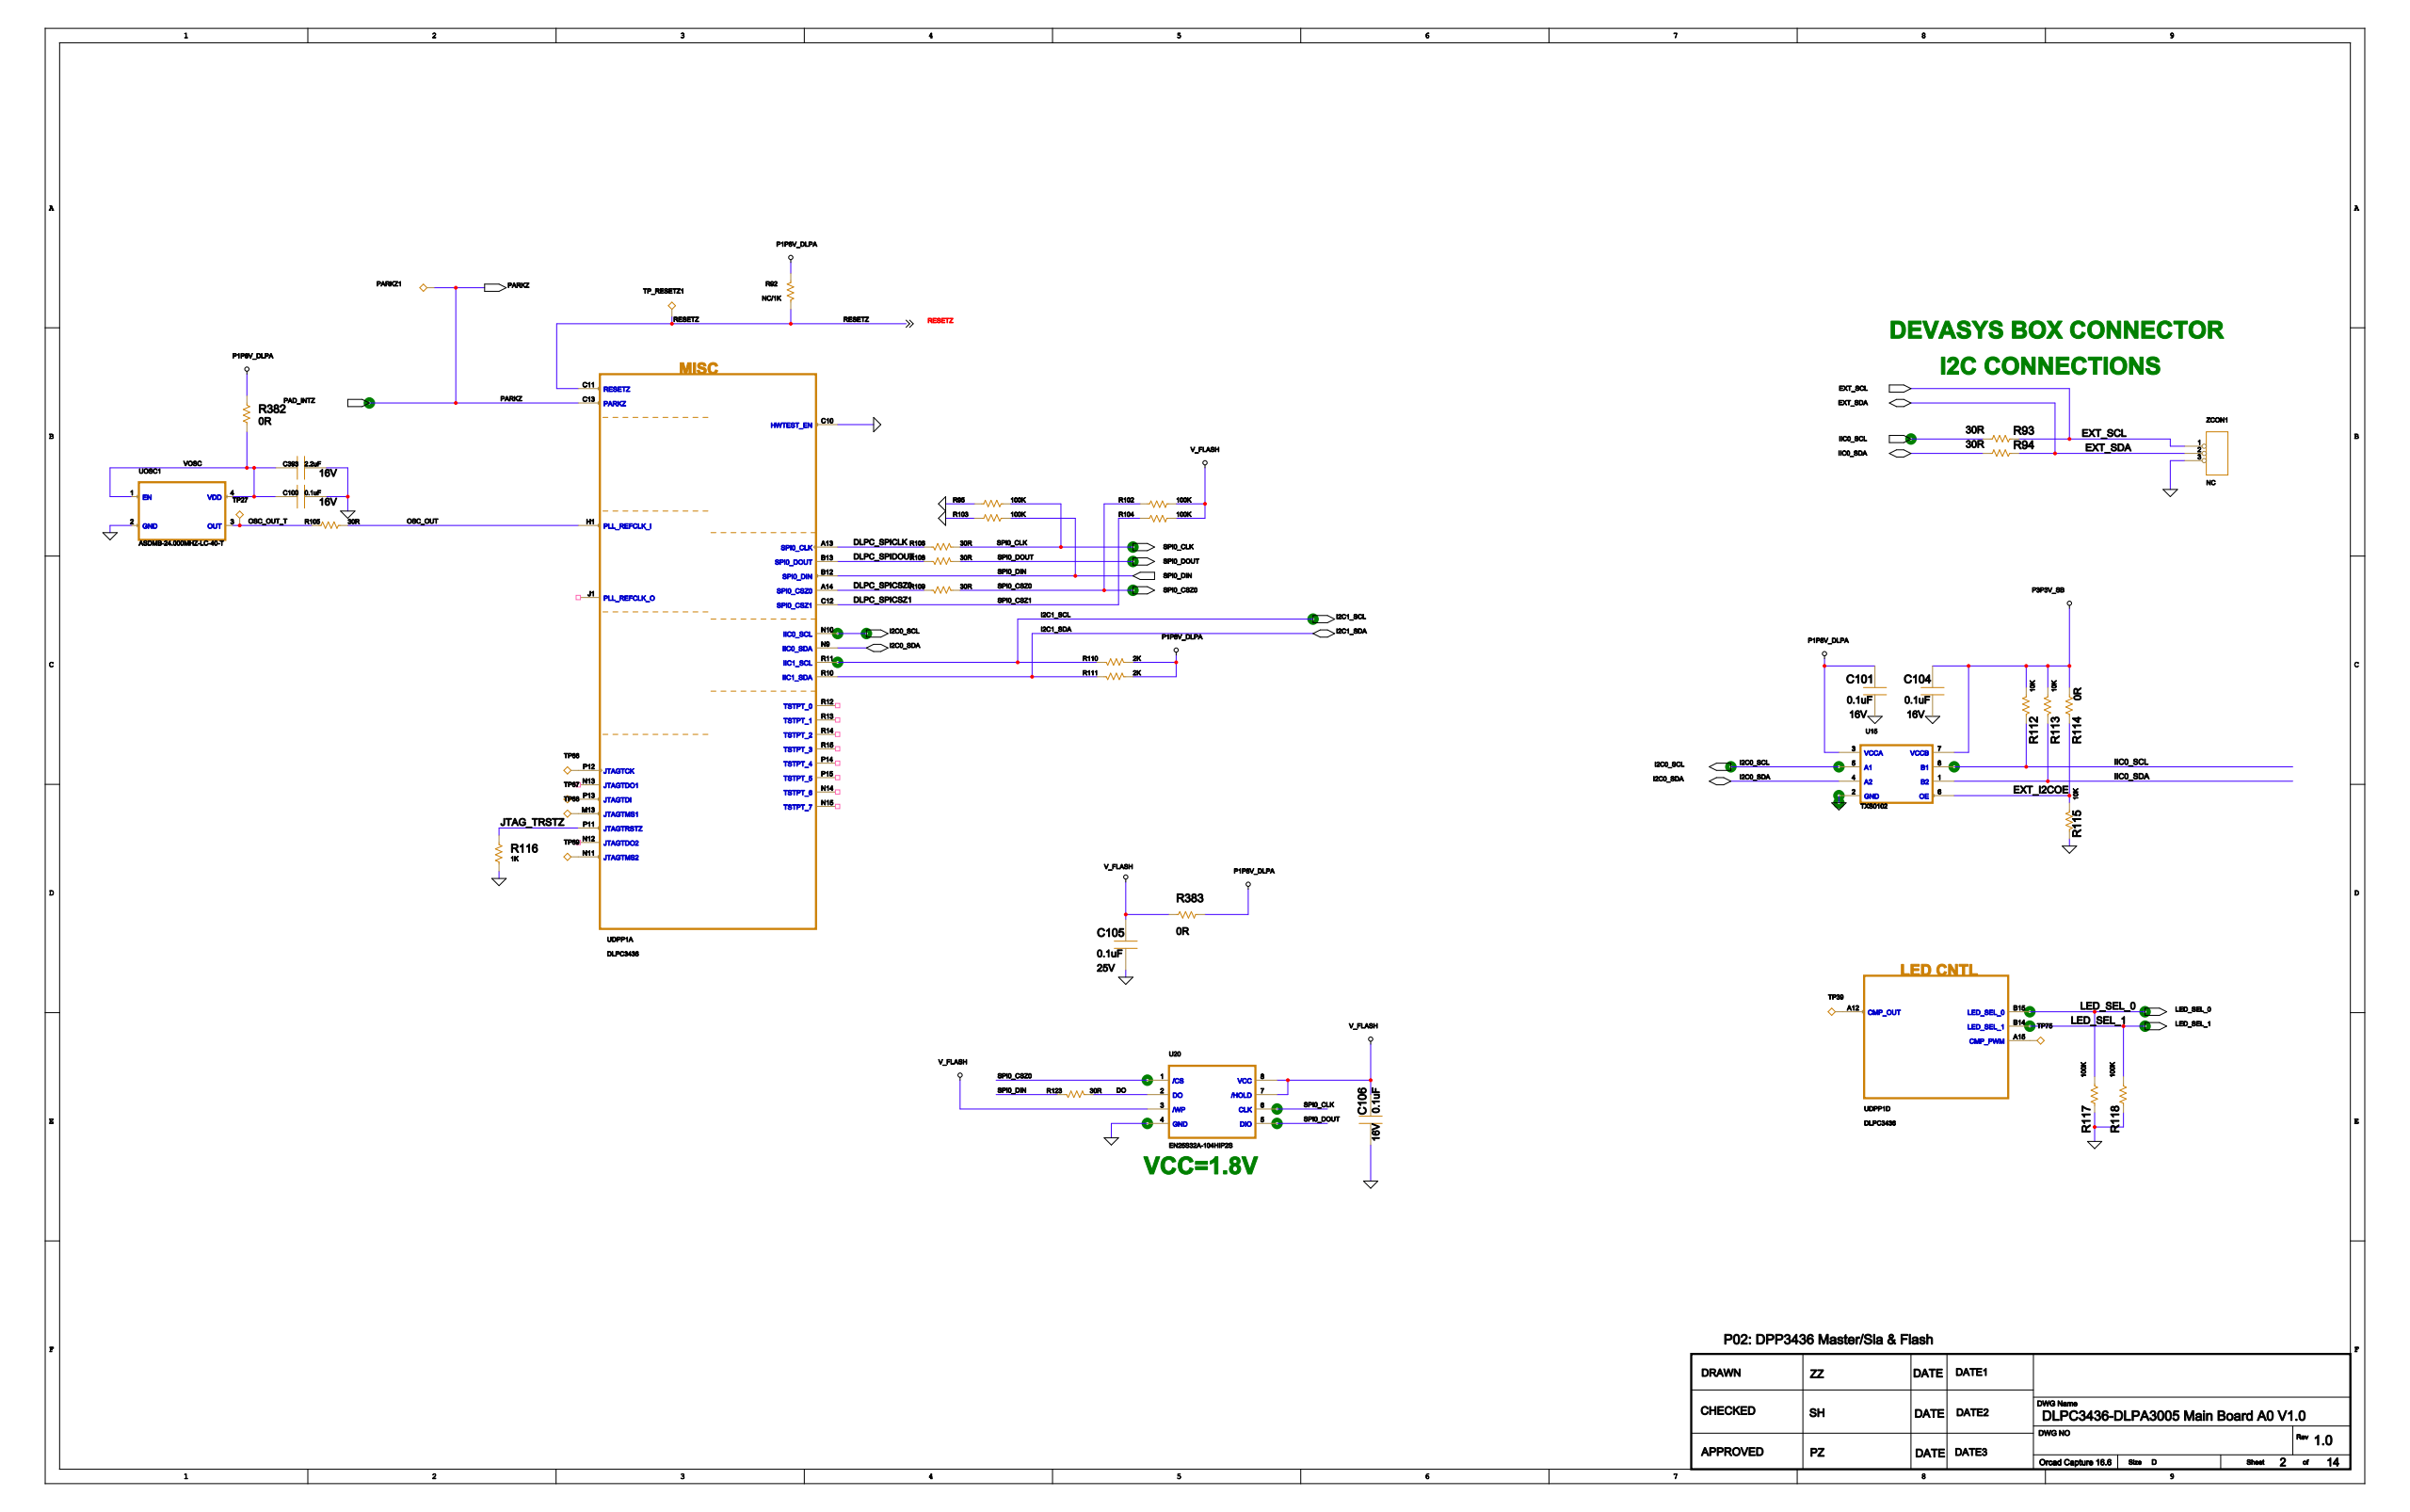Circuit board | Cadence Allegro | 1223 parts | 777 nets | one sheet of the schematic
Parts on this sheet (reference | value | footprint):
C100 | 0.1uF | C0201
C101 | 0.1uF | C0201
C104 | 0.1uF | C0201
C105 | 0.1uF | C0201
C106 | 0.1uF | C0201
C393 | 2.2uF | C0201
PARKZ1 | TP40 | TP06MM
R92 | NC/1K | R0201
R93 | 30R | R0201
R94 | 30R | R0201
R95 | 100K | R0201
R102 | 100K | R0201
R103 | 100K | R0201
R104 | 100K | R0201
R105 | 30R | R0201
R106 | 30R | R0201
R108 | 30R | R0201
R109 | 30R | R0201
R110 | 2K | R0201
R111 | 2K | R0201
R112 | 10K | R0201
R113 | 10K | R0201
R114 | 0R | R0201
R115 | 10K | R0201
R116 | 1K | R0201
R117 | 100K | R0201
R118 | 100K | R0201
R123 | 30R | R0201
R382 | 0R | R0201
R383 | 0R | R0201
TP27 | TP40 | TP06MM
TP39 | TP40 | TP06MM
TP66 | TP40 | TP06MM
TP67 | TP40 | TP06MM
TP68 | TP40 | TP06MM
TP69 | TP40 | TP06MM
TP75 | TP40 | TP06MM
TP_RESETZ1 | TP40 | TP06MM
U15 | TXS0102 | SSOP8_DCU
U20 | EN25S32A-104HIP2S | SOIC-8_208MIL
UDPP1 | DLPC3436 | DLPC3436_176NFBGA
UOSC1 | 24MHz | CRY-D3225
ZCON1 | NC | SIP3
Nets of these parts (net: part-pin ...):
GND: C100-2 C101-2 C104-2 C105-2 C106-2 C393-2 R95-1 R103-1 R115-2 R116-1 R117-1 R118-1 U15-2 U20-4 UOSC1-2 ZCON1-3 UDPP1-C10
VOSC: C100-1 C393-1 R382-1 UOSC1-1 UOSC1-4
P1P8V_DLPA: C101-1 R92-1 R110-1 R111-1 R382-2 R383-1 U15-3
P3P3V_SB: C104-1 R112-1 R113-1 R114-2 U15-7
V_FLASH: C105-1 C106-1 R102-1 R104-1 R383-2 U20-3 U20-7 U20-8
PAD_INTZ: PARKZ1-1 UDPP1-C13
OSC_OUT_T: R105-1 TP27-1 UOSC1-3
N255395943: TP39-1 UDPP1-A12
N255396530: TP66-1 UDPP1-P12
N255396531: TP67-1 UDPP1-P13
N255396532: TP68-1 UDPP1-M13
N2553965326: TP69-1 UDPP1-N11
N255395942: TP75-1 UDPP1-A15
RESETZ: R92-2 TP_RESETZ1-1 UDPP1-C11
SPI0_DIN: R103-2 R123-2 UDPP1-B12
SPI0_CLK: R95-2 R106-1 U20-6
SPI0_DOUT: R108-1 U20-5
SPI0_CSZ0: R102-2 R109-1 U20-1
DLPC_SPICSZ1: R104-2 UDPP1-C12
LED_SEL_0: R117-2 UDPP1-B15
LED_SEL_1: R118-2 UDPP1-B14
OSC_OUT: R105-2 UDPP1-H1
DLPC_SPICLK: R106-2 UDPP1-A13
DLPC_SPIDOUT: R108-2 UDPP1-B13
DLPC_SPICSZ0: R109-2 UDPP1-A14
DO: R123-1 U20-2
IIC0_SCL: R93-1 R112-2 U15-8
EXT_SCL: R93-2 ZCON1-1
IIC0_SDA: R94-1 R113-2 U15-1
EXT_SDA: R94-2 ZCON1-2
I2C1_SCL: R110-2 UDPP1-R11
I2C1_SDA: R111-2 UDPP1-R10
EXT_I2COE: R114-1 R115-1 U15-6
JTAG_TRSTZ: R116-2 UDPP1-P11
I2C0_SCL: U15-5 UDPP1-N10
I2C0_SDA: U15-4 UDPP1-N9